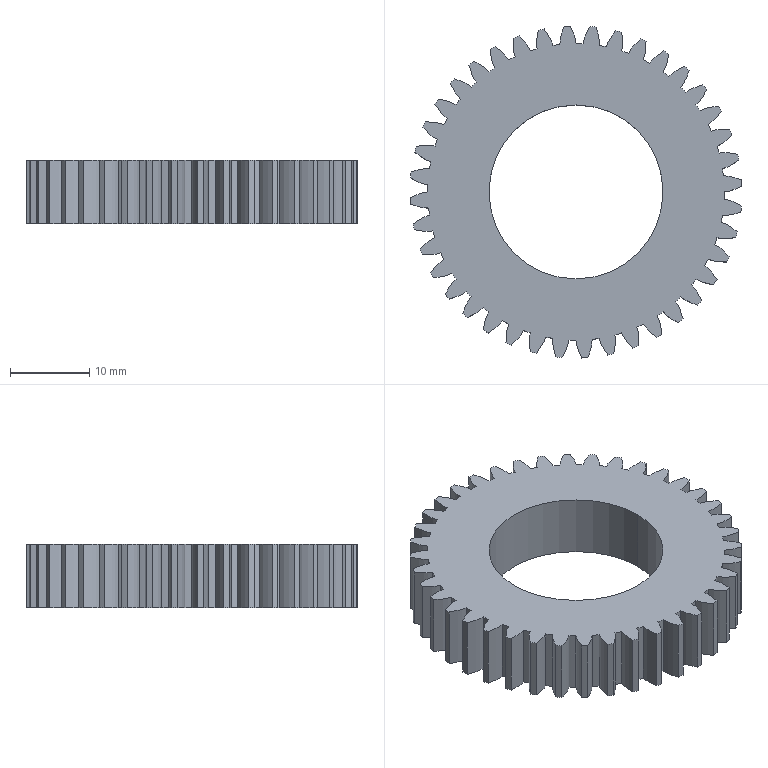Part | SolidWorks | features Boss 1, CirPattern 1, Cut 1, Extrusion 1, RefAxis 1 | 1 solid | 164 faces | box 41.973 x 41.973 x 8 mm | volume 6925 mm3 | cylinder 82 | spline 80 | plane 2 | commonest cylinder face diameters 37.5 x40 42 x40 22 x2